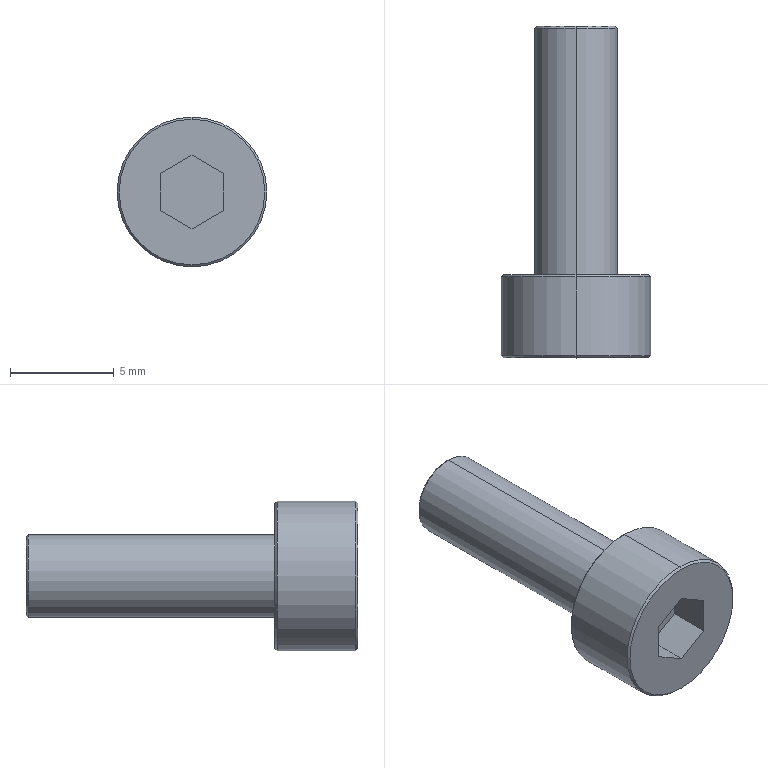Part | SolidWorks | features BaseBody 1 | 1 solid | 20 faces | box 7.22 x 16 x 7.22 mm | volume 297.845 mm3 | plane 10 | cone 6 | cylinder 4 | commonest cylinder face diameters 4 x2 7.22 x2
STEP:
#1=CARTESIAN_POINT('',(0.,15.9,-2.));
#2=VERTEX_POINT('',#1);
#3=CARTESIAN_POINT('',(0.,15.9,2.));
#4=VERTEX_POINT('',#3);
#5=CARTESIAN_POINT('',(0.,15.9,0.));
#6=DIRECTION('',(0.,-1.,0.));
#7=DIRECTION('',(0.,0.,-1.));
#8=AXIS2_PLACEMENT_3D('',#5,#6,#7);
#9=CIRCLE('',#8,2.);
#10=EDGE_CURVE('',#2,#4,#9,.T.);
#11=ORIENTED_EDGE('',*,*,#10,.T.);
#12=CARTESIAN_POINT('',(0.,4.,2.));
#13=VERTEX_POINT('',#12);
#14=CARTESIAN_POINT('',(0.,16.,2.));
#15=DIRECTION('',(0.,-1.,0.));
#16=VECTOR('',#15,1000.);
#17=LINE('',#14,#16);
#18=EDGE_CURVE('',#4,#13,#17,.T.);
#19=ORIENTED_EDGE('',*,*,#18,.T.);
#20=CARTESIAN_POINT('',(0.,4.,-2.));
#21=VERTEX_POINT('',#20);
#22=CARTESIAN_POINT('',(0.,4.,0.));
#23=DIRECTION('',(0.,1.,0.));
#24=DIRECTION('',(0.,0.,-1.));
#25=AXIS2_PLACEMENT_3D('',#22,#23,#24);
#26=CIRCLE('',#25,2.);
#27=EDGE_CURVE('',#13,#21,#26,.T.);
#28=ORIENTED_EDGE('',*,*,#27,.T.);
#29=CARTESIAN_POINT('',(0.,16.,-2.));
#30=DIRECTION('',(0.,-1.,0.));
#31=VECTOR('',#30,1000.);
#32=LINE('',#29,#31);
#33=EDGE_CURVE('',#2,#21,#32,.T.);
#34=ORIENTED_EDGE('',*,*,#33,.F.);
#35=EDGE_LOOP('',(#11,#19,#28,#34));
#36=FACE_OUTER_BOUND('',#35,.T.);
#37=CARTESIAN_POINT('',(0.,16.,0.));
#38=DIRECTION('',(0.,-1.,0.));
#39=DIRECTION('',(0.,0.,-1.));
#40=AXIS2_PLACEMENT_3D('',#37,#38,#39);
#41=CYLINDRICAL_SURFACE('',#40,2.);
#42=ADVANCED_FACE('',(#36),#41,.T.);
#43=CARTESIAN_POINT('',(0.,16.,-1.9));
#44=VERTEX_POINT('',#43);
#45=CARTESIAN_POINT('',(0.,16.,1.9));
#46=VERTEX_POINT('',#45);
#47=CARTESIAN_POINT('',(0.,16.,0.));
#48=DIRECTION('',(0.,-1.,0.));
#49=DIRECTION('',(0.,0.,-1.));
#50=AXIS2_PLACEMENT_3D('',#47,#48,#49);
#51=CIRCLE('',#50,1.9);
#52=EDGE_CURVE('',#44,#46,#51,.T.);
#53=ORIENTED_EDGE('',*,*,#52,.T.);
#54=CARTESIAN_POINT('',(0.,15.9,2.));
#55=DIRECTION('',(0.,-0.7071,0.7071));
#56=VECTOR('',#55,1000.);
#57=LINE('',#54,#56);
#58=EDGE_CURVE('',#46,#4,#57,.T.);
#59=ORIENTED_EDGE('',*,*,#58,.T.);
#60=ORIENTED_EDGE('',*,*,#10,.F.);
#61=CARTESIAN_POINT('',(0.,15.9,-2.));
#62=DIRECTION('',(0.,-0.7071,-0.7071));
#63=VECTOR('',#62,1000.);
#64=LINE('',#61,#63);
#65=EDGE_CURVE('',#44,#2,#64,.T.);
#66=ORIENTED_EDGE('',*,*,#65,.F.);
#67=EDGE_LOOP('',(#53,#59,#60,#66));
#68=FACE_OUTER_BOUND('',#67,.T.);
#69=CARTESIAN_POINT('',(0.,15.9,0.));
#70=DIRECTION('',(0.,-1.,0.));
#71=DIRECTION('',(0.,0.,-1.));
#72=AXIS2_PLACEMENT_3D('',#69,#70,#71);
#73=CONICAL_SURFACE('',#72,2.,0.7854);
#74=ADVANCED_FACE('',(#68),#73,.T.);
#75=CARTESIAN_POINT('',(0.,4.,3.51));
#76=VERTEX_POINT('',#75);
#77=CARTESIAN_POINT('',(0.,4.,-3.51));
#78=VERTEX_POINT('',#77);
#79=CARTESIAN_POINT('',(0.,4.,0.));
#80=DIRECTION('',(0.,1.,0.));
#81=DIRECTION('',(0.,0.,-1.));
#82=AXIS2_PLACEMENT_3D('',#79,#80,#81);
#83=CIRCLE('',#82,3.51);
#84=EDGE_CURVE('',#76,#78,#83,.T.);
#85=ORIENTED_EDGE('',*,*,#84,.F.);
#86=CARTESIAN_POINT('',(0.,3.9,3.61));
#87=VERTEX_POINT('',#86);
#88=CARTESIAN_POINT('',(0.,3.9,3.61));
#89=DIRECTION('',(0.,-0.7071,0.7071));
#90=VECTOR('',#89,1000.);
#91=LINE('',#88,#90);
#92=EDGE_CURVE('',#76,#87,#91,.T.);
#93=ORIENTED_EDGE('',*,*,#92,.T.);
#94=CARTESIAN_POINT('',(0.,3.9,-3.61));
#95=VERTEX_POINT('',#94);
#96=CARTESIAN_POINT('',(0.,3.9,0.));
#97=DIRECTION('',(0.,1.,0.));
#98=DIRECTION('',(0.,0.,-1.));
#99=AXIS2_PLACEMENT_3D('',#96,#97,#98);
#100=CIRCLE('',#99,3.61);
#101=EDGE_CURVE('',#87,#95,#100,.T.);
#102=ORIENTED_EDGE('',*,*,#101,.T.);
#103=CARTESIAN_POINT('',(0.,3.9,-3.61));
#104=DIRECTION('',(0.,-0.7071,-0.7071));
#105=VECTOR('',#104,1000.);
#106=LINE('',#103,#105);
#107=EDGE_CURVE('',#78,#95,#106,.T.);
#108=ORIENTED_EDGE('',*,*,#107,.F.);
#109=EDGE_LOOP('',(#85,#93,#102,#108));
#110=FACE_OUTER_BOUND('',#109,.T.);
#111=CARTESIAN_POINT('',(0.,3.9,0.));
#112=DIRECTION('',(0.,-1.,0.));
#113=DIRECTION('',(0.,0.,-1.));
#114=AXIS2_PLACEMENT_3D('',#111,#112,#113);
#115=CONICAL_SURFACE('',#114,3.61,0.7854);
#116=ADVANCED_FACE('',(#110),#115,.T.);
#117=ORIENTED_EDGE('',*,*,#101,.F.);
#118=CARTESIAN_POINT('',(0.,0.1,3.61));
#119=VERTEX_POINT('',#118);
#120=CARTESIAN_POINT('',(0.,4.,3.61));
#121=DIRECTION('',(0.,-1.,0.));
#122=VECTOR('',#121,1000.);
#123=LINE('',#120,#122);
#124=EDGE_CURVE('',#87,#119,#123,.T.);
#125=ORIENTED_EDGE('',*,*,#124,.T.);
#126=CARTESIAN_POINT('',(0.,0.1,-3.61));
#127=VERTEX_POINT('',#126);
#128=CARTESIAN_POINT('',(0.,0.1,0.));
#129=DIRECTION('',(0.,1.,0.));
#130=DIRECTION('',(0.,0.,-1.));
#131=AXIS2_PLACEMENT_3D('',#128,#129,#130);
#132=CIRCLE('',#131,3.61);
#133=EDGE_CURVE('',#119,#127,#132,.T.);
#134=ORIENTED_EDGE('',*,*,#133,.T.);
#135=CARTESIAN_POINT('',(0.,4.,-3.61));
#136=DIRECTION('',(0.,-1.,0.));
#137=VECTOR('',#136,1000.);
#138=LINE('',#135,#137);
#139=EDGE_CURVE('',#95,#127,#138,.T.);
#140=ORIENTED_EDGE('',*,*,#139,.F.);
#141=EDGE_LOOP('',(#117,#125,#134,#140));
#142=FACE_OUTER_BOUND('',#141,.T.);
#143=CARTESIAN_POINT('',(0.,4.,0.));
#144=DIRECTION('',(0.,-1.,0.));
#145=DIRECTION('',(0.,0.,-1.));
#146=AXIS2_PLACEMENT_3D('',#143,#144,#145);
#147=CYLINDRICAL_SURFACE('',#146,3.61);
#148=ADVANCED_FACE('',(#142),#147,.T.);
#149=CARTESIAN_POINT('',(0.,0.,3.51));
#150=VERTEX_POINT('',#149);
#151=CARTESIAN_POINT('',(0.,0.,-3.51));
#152=VERTEX_POINT('',#151);
#153=CARTESIAN_POINT('',(0.,0.,0.));
#154=DIRECTION('',(0.,1.,0.));
#155=DIRECTION('',(0.,0.,1.));
#156=AXIS2_PLACEMENT_3D('',#153,#154,#155);
#157=CIRCLE('',#156,3.51);
#158=EDGE_CURVE('',#150,#152,#157,.T.);
#159=ORIENTED_EDGE('',*,*,#158,.T.);
#160=CARTESIAN_POINT('',(0.,0.1,-3.61));
#161=DIRECTION('',(0.,0.7071,-0.7071));
#162=VECTOR('',#161,1000.);
#163=LINE('',#160,#162);
#164=EDGE_CURVE('',#152,#127,#163,.T.);
#165=ORIENTED_EDGE('',*,*,#164,.T.);
#166=ORIENTED_EDGE('',*,*,#133,.F.);
#167=CARTESIAN_POINT('',(0.,0.1,3.61));
#168=DIRECTION('',(0.,0.7071,0.7071));
#169=VECTOR('',#168,1000.);
#170=LINE('',#167,#169);
#171=EDGE_CURVE('',#150,#119,#170,.T.);
#172=ORIENTED_EDGE('',*,*,#171,.F.);
#173=EDGE_LOOP('',(#159,#165,#166,#172));
#174=FACE_OUTER_BOUND('',#173,.T.);
#175=CARTESIAN_POINT('',(0.,0.1,0.));
#176=DIRECTION('',(0.,1.,0.));
#177=DIRECTION('',(0.,0.,1.));
#178=AXIS2_PLACEMENT_3D('',#175,#176,#177);
#179=CONICAL_SURFACE('',#178,3.61,0.7854);
#180=ADVANCED_FACE('',(#174),#179,.T.);
#181=ORIENTED_EDGE('',*,*,#18,.F.);
#182=CARTESIAN_POINT('',(0.,15.9,0.));
#183=DIRECTION('',(0.,-1.,0.));
#184=DIRECTION('',(0.,0.,-1.));
#185=AXIS2_PLACEMENT_3D('',#182,#183,#184);
#186=CIRCLE('',#185,2.);
#187=EDGE_CURVE('',#4,#2,#186,.T.);
#188=ORIENTED_EDGE('',*,*,#187,.T.);
#189=ORIENTED_EDGE('',*,*,#33,.T.);
#190=CARTESIAN_POINT('',(0.,4.,0.));
#191=DIRECTION('',(0.,1.,0.));
#192=DIRECTION('',(0.,0.,-1.));
#193=AXIS2_PLACEMENT_3D('',#190,#191,#192);
#194=CIRCLE('',#193,2.);
#195=EDGE_CURVE('',#21,#13,#194,.T.);
#196=ORIENTED_EDGE('',*,*,#195,.T.);
#197=EDGE_LOOP('',(#181,#188,#189,#196));
#198=FACE_OUTER_BOUND('',#197,.T.);
#199=CARTESIAN_POINT('',(0.,16.,0.));
#200=DIRECTION('',(0.,-1.,0.));
#201=DIRECTION('',(0.,0.,-1.));
#202=AXIS2_PLACEMENT_3D('',#199,#200,#201);
#203=CYLINDRICAL_SURFACE('',#202,2.);
#204=ADVANCED_FACE('',(#198),#203,.T.);
#205=ORIENTED_EDGE('',*,*,#195,.F.);
#206=ORIENTED_EDGE('',*,*,#27,.F.);
#207=EDGE_LOOP('',(#205,#206));
#208=FACE_BOUND('',#207,.T.);
#209=CARTESIAN_POINT('',(0.,4.,0.));
#210=DIRECTION('',(0.,1.,0.));
#211=DIRECTION('',(0.,0.,-1.));
#212=AXIS2_PLACEMENT_3D('',#209,#210,#211);
#213=CIRCLE('',#212,3.51);
#214=EDGE_CURVE('',#78,#76,#213,.T.);
#215=ORIENTED_EDGE('',*,*,#214,.T.);
#216=ORIENTED_EDGE('',*,*,#84,.T.);
#217=EDGE_LOOP('',(#215,#216));
#218=FACE_OUTER_BOUND('',#217,.T.);
#219=CARTESIAN_POINT('',(0.,4.,0.));
#220=DIRECTION('',(0.,1.,0.));
#221=DIRECTION('',(0.,0.,1.));
#222=AXIS2_PLACEMENT_3D('',#219,#220,#221);
#223=PLANE('',#222);
#224=ADVANCED_FACE('',(#208,#218),#223,.T.);
#225=ORIENTED_EDGE('',*,*,#58,.F.);
#226=CARTESIAN_POINT('',(0.,16.,0.));
#227=DIRECTION('',(0.,-1.,0.));
#228=DIRECTION('',(0.,0.,-1.));
#229=AXIS2_PLACEMENT_3D('',#226,#227,#228);
#230=CIRCLE('',#229,1.9);
#231=EDGE_CURVE('',#46,#44,#230,.T.);
#232=ORIENTED_EDGE('',*,*,#231,.T.);
#233=ORIENTED_EDGE('',*,*,#65,.T.);
#234=ORIENTED_EDGE('',*,*,#187,.F.);
#235=EDGE_LOOP('',(#225,#232,#233,#234));
#236=FACE_OUTER_BOUND('',#235,.T.);
#237=CARTESIAN_POINT('',(0.,15.9,0.));
#238=DIRECTION('',(0.,-1.,0.));
#239=DIRECTION('',(0.,0.,-1.));
#240=AXIS2_PLACEMENT_3D('',#237,#238,#239);
#241=CONICAL_SURFACE('',#240,2.,0.7854);
#242=ADVANCED_FACE('',(#236),#241,.T.);
#243=ORIENTED_EDGE('',*,*,#92,.F.);
#244=ORIENTED_EDGE('',*,*,#214,.F.);
#245=ORIENTED_EDGE('',*,*,#107,.T.);
#246=CARTESIAN_POINT('',(0.,3.9,0.));
#247=DIRECTION('',(0.,1.,0.));
#248=DIRECTION('',(0.,0.,-1.));
#249=AXIS2_PLACEMENT_3D('',#246,#247,#248);
#250=CIRCLE('',#249,3.61);
#251=EDGE_CURVE('',#95,#87,#250,.T.);
#252=ORIENTED_EDGE('',*,*,#251,.T.);
#253=EDGE_LOOP('',(#243,#244,#245,#252));
#254=FACE_OUTER_BOUND('',#253,.T.);
#255=CARTESIAN_POINT('',(0.,3.9,0.));
#256=DIRECTION('',(0.,-1.,0.));
#257=DIRECTION('',(0.,0.,-1.));
#258=AXIS2_PLACEMENT_3D('',#255,#256,#257);
#259=CONICAL_SURFACE('',#258,3.61,0.7854);
#260=ADVANCED_FACE('',(#254),#259,.T.);
#261=ORIENTED_EDGE('',*,*,#52,.F.);
#262=ORIENTED_EDGE('',*,*,#231,.F.);
#263=EDGE_LOOP('',(#261,#262));
#264=FACE_OUTER_BOUND('',#263,.T.);
#265=CARTESIAN_POINT('',(0.,16.,0.));
#266=DIRECTION('',(0.,1.,0.));
#267=DIRECTION('',(0.,0.,1.));
#268=AXIS2_PLACEMENT_3D('',#265,#266,#267);
#269=PLANE('',#268);
#270=ADVANCED_FACE('',(#264),#269,.T.);
#271=ORIENTED_EDGE('',*,*,#124,.F.);
#272=ORIENTED_EDGE('',*,*,#251,.F.);
#273=ORIENTED_EDGE('',*,*,#139,.T.);
#274=CARTESIAN_POINT('',(0.,0.1,0.));
#275=DIRECTION('',(0.,1.,0.));
#276=DIRECTION('',(0.,0.,-1.));
#277=AXIS2_PLACEMENT_3D('',#274,#275,#276);
#278=CIRCLE('',#277,3.61);
#279=EDGE_CURVE('',#127,#119,#278,.T.);
#280=ORIENTED_EDGE('',*,*,#279,.T.);
#281=EDGE_LOOP('',(#271,#272,#273,#280));
#282=FACE_OUTER_BOUND('',#281,.T.);
#283=CARTESIAN_POINT('',(0.,4.,0.));
#284=DIRECTION('',(0.,-1.,0.));
#285=DIRECTION('',(0.,0.,-1.));
#286=AXIS2_PLACEMENT_3D('',#283,#284,#285);
#287=CYLINDRICAL_SURFACE('',#286,3.61);
#288=ADVANCED_FACE('',(#282),#287,.T.);
#289=ORIENTED_EDGE('',*,*,#164,.F.);
#290=CARTESIAN_POINT('',(0.,0.,0.));
#291=DIRECTION('',(0.,1.,0.));
#292=DIRECTION('',(0.,0.,1.));
#293=AXIS2_PLACEMENT_3D('',#290,#291,#292);
#294=CIRCLE('',#293,3.51);
#295=EDGE_CURVE('',#152,#150,#294,.T.);
#296=ORIENTED_EDGE('',*,*,#295,.T.);
#297=ORIENTED_EDGE('',*,*,#171,.T.);
#298=ORIENTED_EDGE('',*,*,#279,.F.);
#299=EDGE_LOOP('',(#289,#296,#297,#298));
#300=FACE_OUTER_BOUND('',#299,.T.);
#301=CARTESIAN_POINT('',(0.,0.1,0.));
#302=DIRECTION('',(0.,1.,0.));
#303=DIRECTION('',(0.,0.,1.));
#304=AXIS2_PLACEMENT_3D('',#301,#302,#303);
#305=CONICAL_SURFACE('',#304,3.61,0.7854);
#306=ADVANCED_FACE('',(#300),#305,.T.);
#307=CARTESIAN_POINT('',(0.,0.,-1.778));
#308=VERTEX_POINT('',#307);
#309=CARTESIAN_POINT('',(1.54,0.,-0.8891));
#310=VERTEX_POINT('',#309);
#311=CARTESIAN_POINT('',(0.,0.,-1.778));
#312=DIRECTION('',(0.866,0.,0.5));
#313=VECTOR('',#312,1000.);
#314=LINE('',#311,#313);
#315=EDGE_CURVE('',#308,#310,#314,.T.);
#316=ORIENTED_EDGE('',*,*,#315,.F.);
#317=CARTESIAN_POINT('',(-1.54,0.,-0.8891));
#318=VERTEX_POINT('',#317);
#319=CARTESIAN_POINT('',(-1.54,0.,-0.8891));
#320=DIRECTION('',(0.866,0.,-0.5));
#321=VECTOR('',#320,1000.);
#322=LINE('',#319,#321);
#323=EDGE_CURVE('',#318,#308,#322,.T.);
#324=ORIENTED_EDGE('',*,*,#323,.F.);
#325=CARTESIAN_POINT('',(-1.54,0.,0.8891));
#326=VERTEX_POINT('',#325);
#327=CARTESIAN_POINT('',(-1.54,0.,0.));
#328=DIRECTION('',(0.,0.,-1.));
#329=VECTOR('',#328,1000.);
#330=LINE('',#327,#329);
#331=EDGE_CURVE('',#326,#318,#330,.T.);
#332=ORIENTED_EDGE('',*,*,#331,.F.);
#333=CARTESIAN_POINT('',(0.,0.,1.778));
#334=VERTEX_POINT('',#333);
#335=CARTESIAN_POINT('',(0.,0.,1.778));
#336=DIRECTION('',(-0.866,0.,-0.5));
#337=VECTOR('',#336,1000.);
#338=LINE('',#335,#337);
#339=EDGE_CURVE('',#334,#326,#338,.T.);
#340=ORIENTED_EDGE('',*,*,#339,.F.);
#341=CARTESIAN_POINT('',(1.54,0.,0.8891));
#342=VERTEX_POINT('',#341);
#343=CARTESIAN_POINT('',(1.54,0.,0.8891));
#344=DIRECTION('',(-0.866,0.,0.5));
#345=VECTOR('',#344,1000.);
#346=LINE('',#343,#345);
#347=EDGE_CURVE('',#342,#334,#346,.T.);
#348=ORIENTED_EDGE('',*,*,#347,.F.);
#349=CARTESIAN_POINT('',(1.54,0.,0.));
#350=DIRECTION('',(0.,0.,1.));
#351=VECTOR('',#350,1000.);
#352=LINE('',#349,#351);
#353=EDGE_CURVE('',#310,#342,#352,.T.);
#354=ORIENTED_EDGE('',*,*,#353,.F.);
#355=EDGE_LOOP('',(#316,#324,#332,#340,#348,#354));
#356=FACE_BOUND('',#355,.T.);
#357=ORIENTED_EDGE('',*,*,#158,.F.);
#358=ORIENTED_EDGE('',*,*,#295,.F.);
#359=EDGE_LOOP('',(#357,#358));
#360=FACE_OUTER_BOUND('',#359,.T.);
#361=CARTESIAN_POINT('',(0.,0.,0.));
#362=DIRECTION('',(0.,1.,0.));
#363=DIRECTION('',(0.,0.,1.));
#364=AXIS2_PLACEMENT_3D('',#361,#362,#363);
#365=PLANE('',#364);
#366=ADVANCED_FACE('',(#356,#360),#365,.F.);
#367=CARTESIAN_POINT('',(1.54,2.,0.8891));
#368=VERTEX_POINT('',#367);
#369=CARTESIAN_POINT('',(1.54,2.,0.8891));
#370=DIRECTION('',(0.,-1.,0.));
#371=VECTOR('',#370,1000.);
#372=LINE('',#369,#371);
#373=EDGE_CURVE('',#368,#342,#372,.T.);
#374=ORIENTED_EDGE('',*,*,#373,.F.);
#375=CARTESIAN_POINT('',(1.54,2.,-0.8891));
#376=VERTEX_POINT('',#375);
#377=CARTESIAN_POINT('',(1.54,2.,-0.8891));
#378=DIRECTION('',(0.,0.,1.));
#379=VECTOR('',#378,1000.);
#380=LINE('',#377,#379);
#381=EDGE_CURVE('',#376,#368,#380,.T.);
#382=ORIENTED_EDGE('',*,*,#381,.F.);
#383=CARTESIAN_POINT('',(1.54,2.,-0.8891));
#384=DIRECTION('',(0.,1.,0.));
#385=VECTOR('',#384,1000.);
#386=LINE('',#383,#385);
#387=EDGE_CURVE('',#310,#376,#386,.T.);
#388=ORIENTED_EDGE('',*,*,#387,.F.);
#389=ORIENTED_EDGE('',*,*,#353,.T.);
#390=EDGE_LOOP('',(#374,#382,#388,#389));
#391=FACE_OUTER_BOUND('',#390,.T.);
#392=CARTESIAN_POINT('',(1.54,2.,-0.8891));
#393=DIRECTION('',(1.,0.,0.));
#394=DIRECTION('',(0.,0.,-1.));
#395=AXIS2_PLACEMENT_3D('',#392,#393,#394);
#396=PLANE('',#395);
#397=ADVANCED_FACE('',(#391),#396,.F.);
#398=ORIENTED_EDGE('',*,*,#387,.T.);
#399=CARTESIAN_POINT('',(0.,2.,-1.778));
#400=VERTEX_POINT('',#399);
#401=CARTESIAN_POINT('',(0.,2.,-1.778));
#402=DIRECTION('',(0.866,0.,0.5));
#403=VECTOR('',#402,1000.);
#404=LINE('',#401,#403);
#405=EDGE_CURVE('',#400,#376,#404,.T.);
#406=ORIENTED_EDGE('',*,*,#405,.F.);
#407=CARTESIAN_POINT('',(0.,2.,-1.778));
#408=DIRECTION('',(0.,1.,0.));
#409=VECTOR('',#408,1000.);
#410=LINE('',#407,#409);
#411=EDGE_CURVE('',#308,#400,#410,.T.);
#412=ORIENTED_EDGE('',*,*,#411,.F.);
#413=ORIENTED_EDGE('',*,*,#315,.T.);
#414=EDGE_LOOP('',(#398,#406,#412,#413));
#415=FACE_OUTER_BOUND('',#414,.T.);
#416=CARTESIAN_POINT('',(0.,2.,-1.778));
#417=DIRECTION('',(0.5,0.,-0.866));
#418=DIRECTION('',(-0.866,0.,-0.5));
#419=AXIS2_PLACEMENT_3D('',#416,#417,#418);
#420=PLANE('',#419);
#421=ADVANCED_FACE('',(#415),#420,.F.);
#422=ORIENTED_EDGE('',*,*,#411,.T.);
#423=CARTESIAN_POINT('',(-1.54,2.,-0.8891));
#424=VERTEX_POINT('',#423);
#425=CARTESIAN_POINT('',(-1.54,2.,-0.8891));
#426=DIRECTION('',(0.866,0.,-0.5));
#427=VECTOR('',#426,1000.);
#428=LINE('',#425,#427);
#429=EDGE_CURVE('',#424,#400,#428,.T.);
#430=ORIENTED_EDGE('',*,*,#429,.F.);
#431=CARTESIAN_POINT('',(-1.54,2.,-0.8891));
#432=DIRECTION('',(0.,1.,0.));
#433=VECTOR('',#432,1000.);
#434=LINE('',#431,#433);
#435=EDGE_CURVE('',#318,#424,#434,.T.);
#436=ORIENTED_EDGE('',*,*,#435,.F.);
#437=ORIENTED_EDGE('',*,*,#323,.T.);
#438=EDGE_LOOP('',(#422,#430,#436,#437));
#439=FACE_OUTER_BOUND('',#438,.T.);
#440=CARTESIAN_POINT('',(-1.54,2.,-0.8891));
#441=DIRECTION('',(-0.5,0.,-0.866));
#442=DIRECTION('',(-0.866,0.,0.5));
#443=AXIS2_PLACEMENT_3D('',#440,#441,#442);
#444=PLANE('',#443);
#445=ADVANCED_FACE('',(#439),#444,.F.);
#446=ORIENTED_EDGE('',*,*,#435,.T.);
#447=CARTESIAN_POINT('',(-1.54,2.,0.8891));
#448=VERTEX_POINT('',#447);
#449=CARTESIAN_POINT('',(-1.54,2.,0.8891));
#450=DIRECTION('',(0.,0.,-1.));
#451=VECTOR('',#450,1000.);
#452=LINE('',#449,#451);
#453=EDGE_CURVE('',#448,#424,#452,.T.);
#454=ORIENTED_EDGE('',*,*,#453,.F.);
#455=CARTESIAN_POINT('',(-1.54,2.,0.8891));
#456=DIRECTION('',(0.,1.,0.));
#457=VECTOR('',#456,1000.);
#458=LINE('',#455,#457);
#459=EDGE_CURVE('',#326,#448,#458,.T.);
#460=ORIENTED_EDGE('',*,*,#459,.F.);
#461=ORIENTED_EDGE('',*,*,#331,.T.);
#462=EDGE_LOOP('',(#446,#454,#460,#461));
#463=FACE_OUTER_BOUND('',#462,.T.);
#464=CARTESIAN_POINT('',(-1.54,2.,0.8891));
#465=DIRECTION('',(-1.,0.,0.));
#466=DIRECTION('',(0.,0.,1.));
#467=AXIS2_PLACEMENT_3D('',#464,#465,#466);
#468=PLANE('',#467);
#469=ADVANCED_FACE('',(#463),#468,.F.);
#470=ORIENTED_EDGE('',*,*,#459,.T.);
#471=CARTESIAN_POINT('',(0.,2.,1.778));
#472=VERTEX_POINT('',#471);
#473=CARTESIAN_POINT('',(0.,2.,1.778));
#474=DIRECTION('',(-0.866,0.,-0.5));
#475=VECTOR('',#474,1000.);
#476=LINE('',#473,#475);
#477=EDGE_CURVE('',#472,#448,#476,.T.);
#478=ORIENTED_EDGE('',*,*,#477,.F.);
#479=CARTESIAN_POINT('',(0.,2.,1.778));
#480=DIRECTION('',(0.,1.,0.));
#481=VECTOR('',#480,1000.);
#482=LINE('',#479,#481);
#483=EDGE_CURVE('',#334,#472,#482,.T.);
#484=ORIENTED_EDGE('',*,*,#483,.F.);
#485=ORIENTED_EDGE('',*,*,#339,.T.);
#486=EDGE_LOOP('',(#470,#478,#484,#485));
#487=FACE_OUTER_BOUND('',#486,.T.);
#488=CARTESIAN_POINT('',(0.,2.,1.778));
#489=DIRECTION('',(-0.5,0.,0.866));
#490=DIRECTION('',(0.866,0.,0.5));
#491=AXIS2_PLACEMENT_3D('',#488,#489,#490);
#492=PLANE('',#491);
#493=ADVANCED_FACE('',(#487),#492,.F.);
#494=ORIENTED_EDGE('',*,*,#483,.T.);
#495=CARTESIAN_POINT('',(1.54,2.,0.8891));
#496=DIRECTION('',(-0.866,0.,0.5));
#497=VECTOR('',#496,1000.);
#498=LINE('',#495,#497);
#499=EDGE_CURVE('',#368,#472,#498,.T.);
#500=ORIENTED_EDGE('',*,*,#499,.F.);
#501=ORIENTED_EDGE('',*,*,#373,.T.);
#502=ORIENTED_EDGE('',*,*,#347,.T.);
#503=EDGE_LOOP('',(#494,#500,#501,#502));
#504=FACE_OUTER_BOUND('',#503,.T.);
#505=CARTESIAN_POINT('',(1.54,2.,0.8891));
#506=DIRECTION('',(0.5,0.,0.866));
#507=DIRECTION('',(0.866,0.,-0.5));
#508=AXIS2_PLACEMENT_3D('',#505,#506,#507);
#509=PLANE('',#508);
#510=ADVANCED_FACE('',(#504),#509,.F.);
#511=ORIENTED_EDGE('',*,*,#453,.T.);
#512=ORIENTED_EDGE('',*,*,#429,.T.);
#513=ORIENTED_EDGE('',*,*,#405,.T.);
#514=ORIENTED_EDGE('',*,*,#381,.T.);
#515=ORIENTED_EDGE('',*,*,#499,.T.);
#516=ORIENTED_EDGE('',*,*,#477,.T.);
#517=EDGE_LOOP('',(#511,#512,#513,#514,#515,#516));
#518=FACE_OUTER_BOUND('',#517,.T.);
#519=CARTESIAN_POINT('',(0.,2.,0.));
#520=DIRECTION('',(0.,-1.,0.));
#521=DIRECTION('',(0.,0.,-1.));
#522=AXIS2_PLACEMENT_3D('',#519,#520,#521);
#523=PLANE('',#522);
#524=ADVANCED_FACE('',(#518),#523,.T.);
#525=CLOSED_SHELL('',(#42,#74,#116,#148,#180,#204,#224,#242,#260,#270,#288,#306,#366,#397,#421,#445,#469,#493,#510,#524));
#526=MANIFOLD_SOLID_BREP('',#525);
#527=CARTESIAN_POINT('',(0.,0.,0.));
#528=DIRECTION('',(0.,0.,1.));
#529=DIRECTION('',(1.,0.,0.));
#530=AXIS2_PLACEMENT_3D('',#527,#528,#529);
#531=(LENGTH_UNIT()NAMED_UNIT(*)SI_UNIT(.MILLI.,.METRE.));
#532=UNCERTAINTY_MEASURE_WITH_UNIT(LENGTH_MEASURE(0.00001),#531,'','');
#533=(NAMED_UNIT(*)PLANE_ANGLE_UNIT()SI_UNIT($,.RADIAN.));
#534=(NAMED_UNIT(*)SI_UNIT($,.STERADIAN.)SOLID_ANGLE_UNIT());
#535=(GEOMETRIC_REPRESENTATION_CONTEXT(3)GLOBAL_UNCERTAINTY_ASSIGNED_CONTEXT((#532))GLOBAL_UNIT_ASSIGNED_CONTEXT((#531,#533,#534))REPRESENTATION_CONTEXT('',''));
#536=ADVANCED_BREP_SHAPE_REPRESENTATION('',(#526,#530),#535);